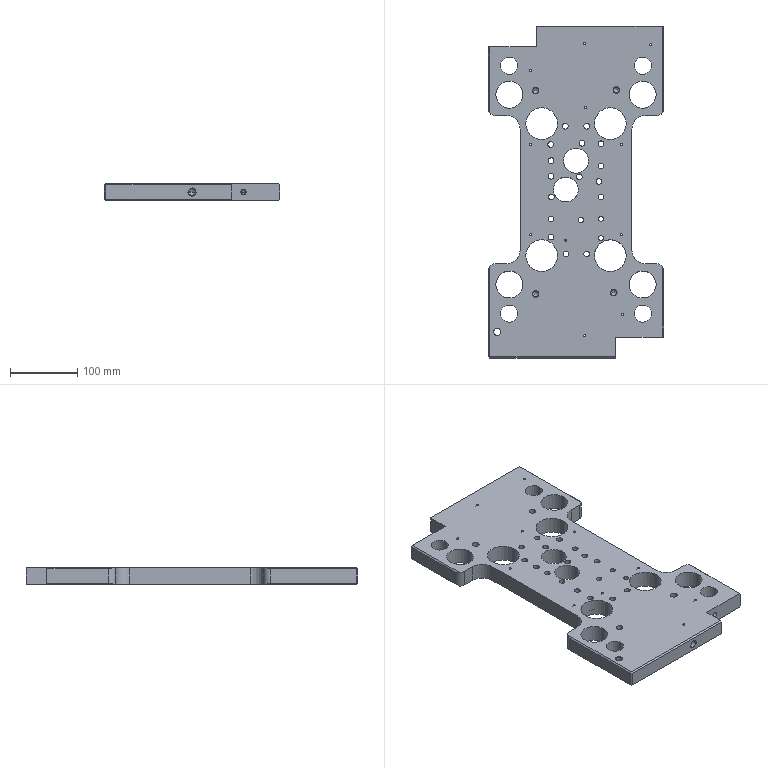Part | Creo | 1 solid | 473 faces | box 260 x 493 x 25 mm | volume 2091396 mm3 | cylinder 206 | plane 121 | other 74 | cone 72 | commonest cylinder face diameters 8.5 x32 12 x30 10.2 x26 14 x26 10 x16 40 x12